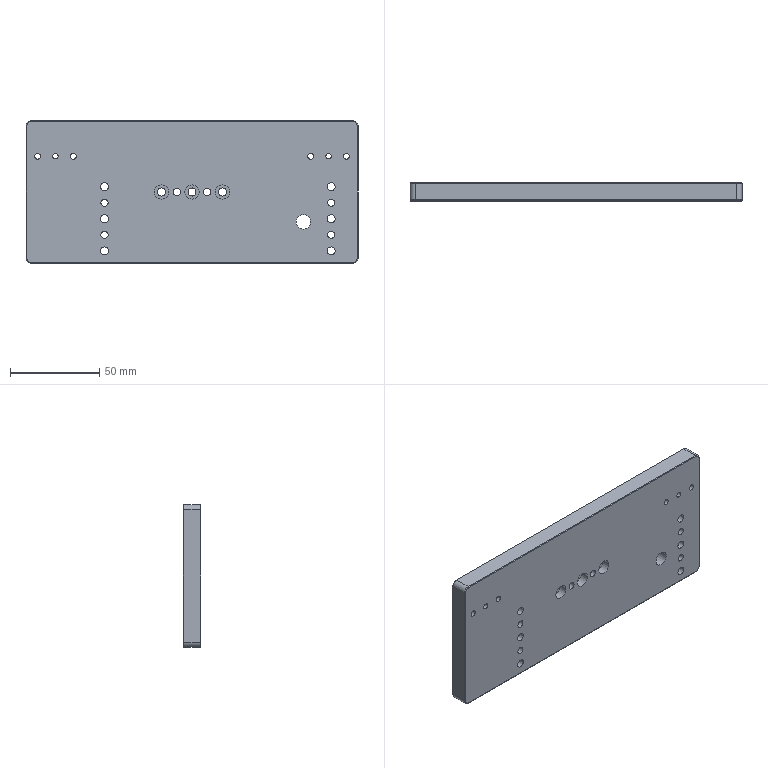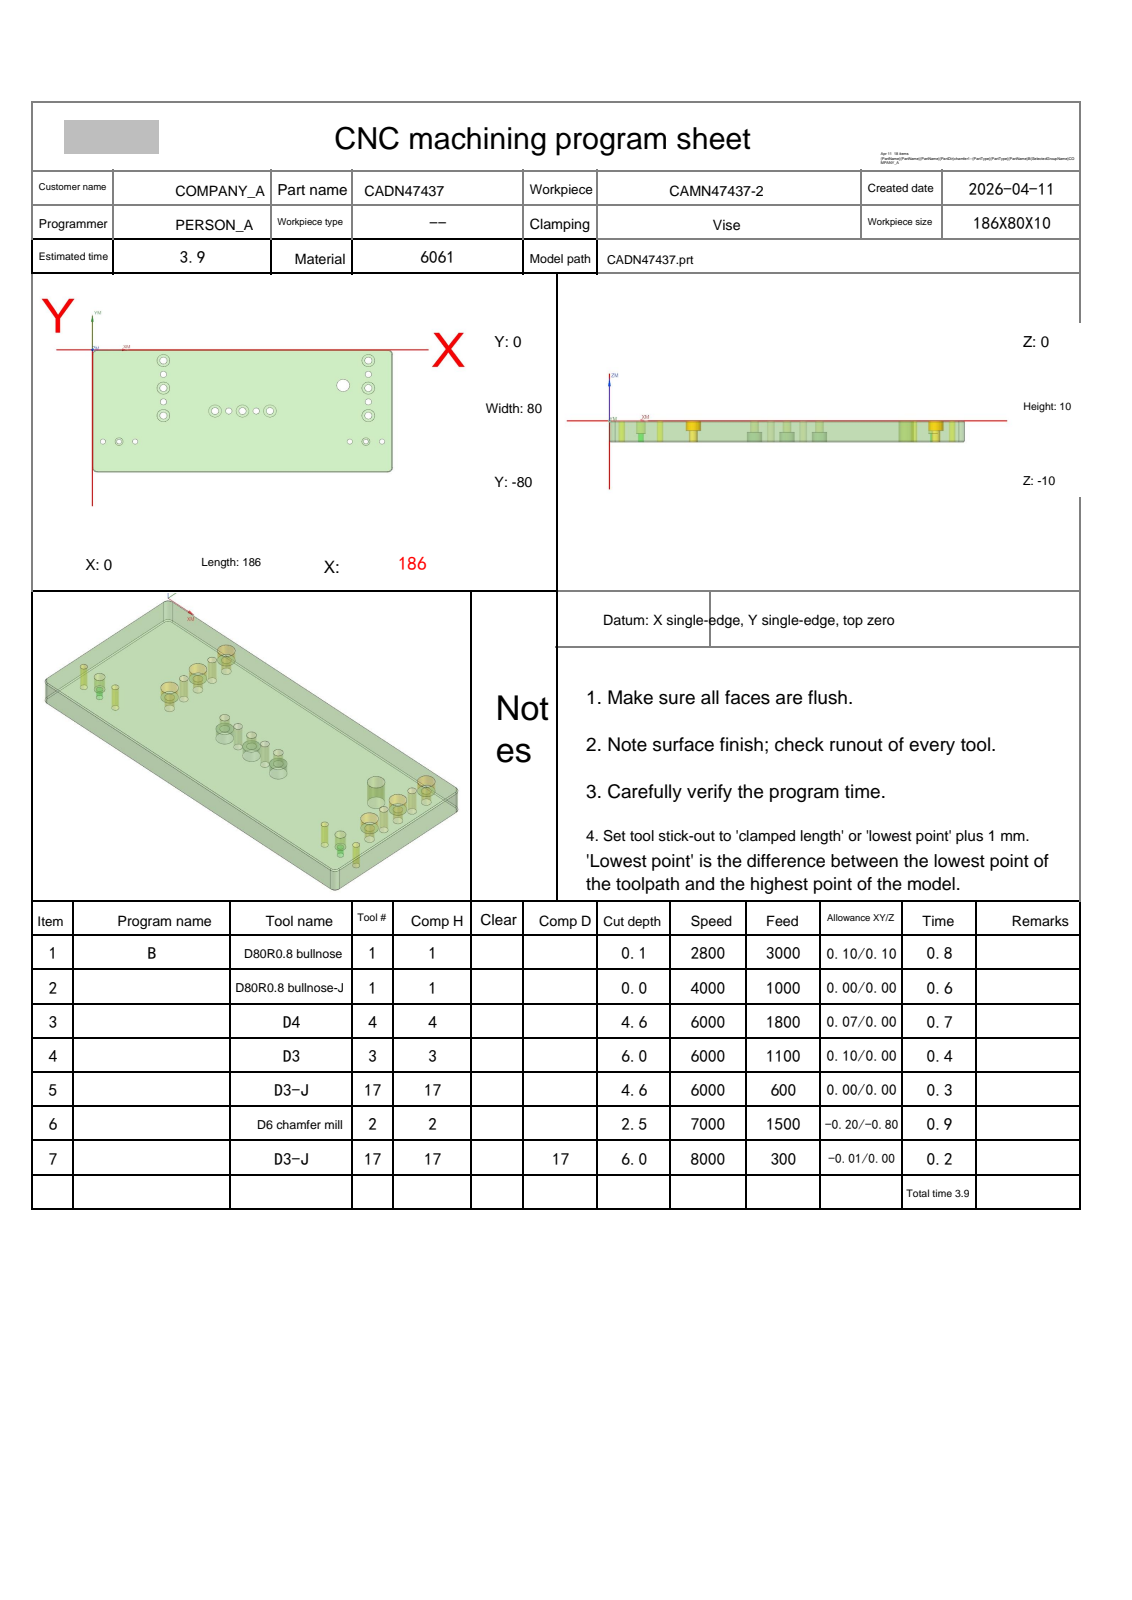NC program | NX | posted by the shop | part box 186 x 10 x 80 mm
Whole program:
%
O0001
(Machine time: 5.17 MIN)
(===Total Tool:5===)
(T1=D80R0.8 bullnose D=80.  R=0.8  D-  H01 Z=0.    )
(T4=D4      D=4.   R=0.   D-  H04 Z=-4.6  )
(T3=D3      D=3.   R=0.   D-  H03 Z=-6.   )
(T17=D3-J   D=3.   R=0.   D-  H17 Z=-6.   )
(T2=D6 chamfer mill   D=6.   R=0.   D-  H02 Z=-2.45 )
G80 G90 G17 G49 G40
G91 G28 Z0
M01
N1 T01 M06
(D80R0.8 bullnose  D=80. R=0.8 H=01 ce=0.10 di=0.10)
G00 G90 G54 X238.097 Y-55.279 M03 S2800
G43 H01 Z20.
M08
Z3.525
G01 Z1.525 F3000.
X226.097 Y-55.457
X-32.79 Y-59.288
X-32.897 Y-59.289
G02 X-40.097 Y-52.089 I0.0 J7.2
G01 Y-39.787
G02 X-32.215 Y-31.788 I8. J0.0
G01 X226.097 Y-27.964
X238.097 Y-27.787
Z3.525
G00 Y-55.279
Z3.05
G01 Z1.05
X226.097 Y-55.457
X-32.79 Y-59.288
X-32.897 Y-59.289
G02 X-40.097 Y-52.089 I0.0 J7.2
G01 Y-39.787
G02 X-32.215 Y-31.788 I8. J0.0
G01 X226.097 Y-27.964
X238.097 Y-27.787
Z3.05
G00 Y-55.279
Z2.575
G01 Z.575
X226.097 Y-55.457
X-32.79 Y-59.288
X-32.897 Y-59.289
G02 X-40.097 Y-52.089 I0.0 J7.2
G01 Y-39.787
G02 X-32.215 Y-31.788 I8. J0.0
G01 X226.097 Y-27.964
X238.097 Y-27.787
Z2.575
G00 Y-55.279
Z2.1
G01 Z.1
X226.097 Y-55.457
X-32.79 Y-59.288
X-32.897 Y-59.289
G02 X-40.097 Y-52.089 I0.0 J7.2
G01 Y-39.787
G02 X-32.215 Y-31.788 I8. J0.0
G01 X226.097 Y-27.964
X238.097 Y-27.787
Z2.1
G00 Z20.
G91 G28 Z0.0
M05
M09
G91 G28 Z0.0
M01
N2 T01 M06
(D80R0.8 bullnose-J  D=80. R=0.8 H=01 ce=0.00 di=0.00)
G00 G90 G54 X237.999 Y-55.182 M03 S4000
G43 H01 Z20.
M08
Z2.
G01 Z0.0 F1000.
X225.999 Y-55.359
X-32.692 Y-59.193
X-32.799
G02 X-39.999 Y-51.993 I0.0 J7.2
G01 Y-39.884
G02 X-32.118 Y-31.885 I8. J0.0
G01 X225.999 Y-28.06
X237.999 Y-27.882
Z2.
G00 Z20.
G91 G28 Z0.0
M05
M09
G91 G28 Z0.0
M01
N3 T04 M06
(D4  D=4. R=0. H=04 ce=0.07 di=0.00)
G00 G90 G54 X171. Y-25. M03 S6000
G43 H04 Z20.
M08
Z.3
G03 X171.965 Y-25.965 I.965 J0.0 F1800.
X172.93 Y-25. I0.0 J.965
X172.93 Y-25. Z-.05 I-1.93 J0.0
X172.93 Y-25. Z-.4 I-1.93 J0.0
X172.93 Y-25. Z-.75 I-1.93 J0.0
X172.93 Y-25. Z-1.1 I-1.93 J0.0
X172.93 Y-25. Z-1.45 I-1.93 J0.0
X172.93 Y-25. Z-1.8 I-1.93 J0.0
X172.93 Y-25. Z-2.15 I-1.93 J0.0
X172.93 Y-25. Z-2.5 I-1.93 J0.0
X172.93 Y-25. Z-2.85 I-1.93 J0.0
X172.93 Y-25. Z-3.2 I-1.93 J0.0
X172.93 Y-25. Z-3.55 I-1.93 J0.0
X172.93 Y-25. Z-3.9 I-1.93 J0.0
X172.93 Y-25. Z-4.25 I-1.93 J0.0
X172.93 Y-25. Z-4.6 I-1.93 J0.0
X171. Y-23.07 I-1.93 J0.0
X169.07 Y-25. I0.0 J-1.93
X171. Y-26.93 I1.93 J0.0
X172.93 Y-25. I0.0 J1.93
X171.965 Y-24.035 I-.965 J0.0
X171. Y-25. I0.0 J-.965
G00 Z20.
Y-43.
Z.3
G03 X171.965 Y-43.965 I.965 J0.0
X172.93 Y-43. I0.0 J.965
X172.93 Y-43. Z-.05 I-1.93 J0.0
X172.93 Y-43. Z-.4 I-1.93 J0.0
X172.93 Y-43. Z-.75 I-1.93 J0.0
X172.93 Y-43. Z-1.1 I-1.93 J0.0
X172.93 Y-43. Z-1.45 I-1.93 J0.0
X172.93 Y-43. Z-1.8 I-1.93 J0.0
X172.93 Y-43. Z-2.15 I-1.93 J0.0
X172.93 Y-43. Z-2.5 I-1.93 J0.0
X172.93 Y-43. Z-2.85 I-1.93 J0.0
X172.93 Y-43. Z-3.2 I-1.93 J0.0
X172.93 Y-43. Z-3.55 I-1.93 J0.0
X172.93 Y-43. Z-3.9 I-1.93 J0.0
X172.93 Y-43. Z-4.25 I-1.93 J0.0
X172.93 Y-43. Z-4.6 I-1.93 J0.0
X171. Y-41.07 I-1.93 J0.0
X169.07 Y-43. I0.0 J-1.93
X171. Y-44.93 I1.93 J0.0
X172.93 Y-43. I0.0 J1.93
X171.965 Y-42.035 I-.965 J0.0
X171. Y-43. I0.0 J-.965
G00 Z20.
Y-7.
Z.3
G03 X171.965 Y-7.965 I.965 J0.0
X172.93 Y-7. I0.0 J.965
X172.93 Y-7. Z-.05 I-1.93 J0.0
X172.93 Y-7. Z-.4 I-1.93 J0.0
X172.93 Y-7. Z-.75 I-1.93 J0.0
X172.93 Y-7. Z-1.1 I-1.93 J0.0
X172.93 Y-7. Z-1.45 I-1.93 J0.0
X172.93 Y-7. Z-1.8 I-1.93 J0.0
X172.93 Y-7. Z-2.15 I-1.93 J0.0
X172.93 Y-7. Z-2.5 I-1.93 J0.0
X172.93 Y-7. Z-2.85 I-1.93 J0.0
X172.93 Y-7. Z-3.2 I-1.93 J0.0
X172.93 Y-7. Z-3.55 I-1.93 J0.0
X172.93 Y-7. Z-3.9 I-1.93 J0.0
X172.93 Y-7. Z-4.25 I-1.93 J0.0
X172.93 Y-7. Z-4.6 I-1.93 J0.0
X171. Y-5.07 I-1.93 J0.0
X169.07 Y-7. I0.0 J-1.93
X171. Y-8.93 I1.93 J0.0
X172.93 Y-7. I0.0 J1.93
X171.965 Y-6.035 I-.965 J0.0
X171. Y-7. I0.0 J-.965
G00 Z20.
X44.
Z.3
G03 X44.965 Y-7.965 I.965 J0.0
X45.93 Y-7. I0.0 J.965
X45.93 Y-7. Z-.05 I-1.93 J0.0
X45.93 Y-7. Z-.4 I-1.93 J0.0
X45.93 Y-7. Z-.75 I-1.93 J0.0
X45.93 Y-7. Z-1.1 I-1.93 J0.0
X45.93 Y-7. Z-1.45 I-1.93 J0.0
X45.93 Y-7. Z-1.8 I-1.93 J0.0
X45.93 Y-7. Z-2.15 I-1.93 J0.0
X45.93 Y-7. Z-2.5 I-1.93 J0.0
X45.93 Y-7. Z-2.85 I-1.93 J0.0
X45.93 Y-7. Z-3.2 I-1.93 J0.0
X45.93 Y-7. Z-3.55 I-1.93 J0.0
X45.93 Y-7. Z-3.9 I-1.93 J0.0
X45.93 Y-7. Z-4.25 I-1.93 J0.0
X45.93 Y-7. Z-4.6 I-1.93 J0.0
X44. Y-5.07 I-1.93 J0.0
X42.07 Y-7. I0.0 J-1.93
X44. Y-8.93 I1.93 J0.0
X45.93 Y-7. I0.0 J1.93
X44.965 Y-6.035 I-.965 J0.0
X44. Y-7. I0.0 J-.965
G00 Z20.
Y-25.
Z.3
G03 X44.965 Y-25.965 I.965 J0.0
X45.93 Y-25. I0.0 J.965
X45.93 Y-25. Z-.05 I-1.93 J0.0
X45.93 Y-25. Z-.4 I-1.93 J0.0
X45.93 Y-25. Z-.75 I-1.93 J0.0
X45.93 Y-25. Z-1.1 I-1.93 J0.0
X45.93 Y-25. Z-1.45 I-1.93 J0.0
X45.93 Y-25. Z-1.8 I-1.93 J0.0
X45.93 Y-25. Z-2.15 I-1.93 J0.0
X45.93 Y-25. Z-2.5 I-1.93 J0.0
X45.93 Y-25. Z-2.85 I-1.93 J0.0
X45.93 Y-25. Z-3.2 I-1.93 J0.0
X45.93 Y-25. Z-3.55 I-1.93 J0.0
X45.93 Y-25. Z-3.9 I-1.93 J0.0
X45.93 Y-25. Z-4.25 I-1.93 J0.0
X45.93 Y-25. Z-4.6 I-1.93 J0.0
X44. Y-23.07 I-1.93 J0.0
X42.07 Y-25. I0.0 J-1.93
X44. Y-26.93 I1.93 J0.0
X45.93 Y-25. I0.0 J1.93
X44.965 Y-24.035 I-.965 J0.0
X44. Y-25. I0.0 J-.965
G00 Z20.
Y-43.
Z.3
G03 X44.965 Y-43.965 I.965 J0.0
X45.93 Y-43. I0.0 J.965
X45.93 Y-43. Z-.05 I-1.93 J0.0
X45.93 Y-43. Z-.4 I-1.93 J0.0
X45.93 Y-43. Z-.75 I-1.93 J0.0
X45.93 Y-43. Z-1.1 I-1.93 J0.0
X45.93 Y-43. Z-1.45 I-1.93 J0.0
X45.93 Y-43. Z-1.8 I-1.93 J0.0
X45.93 Y-43. Z-2.15 I-1.93 J0.0
X45.93 Y-43. Z-2.5 I-1.93 J0.0
X45.93 Y-43. Z-2.85 I-1.93 J0.0
X45.93 Y-43. Z-3.2 I-1.93 J0.0
X45.93 Y-43. Z-3.55 I-1.93 J0.0
X45.93 Y-43. Z-3.9 I-1.93 J0.0
X45.93 Y-43. Z-4.25 I-1.93 J0.0
X45.93 Y-43. Z-4.6 I-1.93 J0.0
X44. Y-41.07 I-1.93 J0.0
X42.07 Y-43. I0.0 J-1.93
X44. Y-44.93 I1.93 J0.0
X45.93 Y-43. I0.0 J1.93
X44.965 Y-42.035 I-.965 J0.0
X44. Y-43. I0.0 J-.965
G00 Z20.
G91 G28 Z0.0
M05
M09
G91 G28 Z0.0
M01
N4 T03 M06
(D3  D=3. R=0. H=03 ce=0.10 di=0.00)
G00 G90 G54 X169.5 Y-60. M03 S6000
G43 H03 Z20.
M08
Z.3
G03 X169.95 Y-60.45 I.45 J0.0 F1100.
X170.4 Y-60. I0.0 J.45
X170.4 Y-60. Z.1 I-.9 J0.0
X170.4 Y-60. Z-.1 I-.9 J0.0
X170.4 Y-60. Z-.3 I-.9 J0.0
X170.4 Y-60. Z-.5 I-.9 J0.0
X170.4 Y-60. Z-.7 I-.9 J0.0
X170.4 Y-60. Z-.9 I-.9 J0.0
X170.4 Y-60. Z-1.1 I-.9 J0.0
X170.4 Y-60. Z-1.3 I-.9 J0.0
X170.4 Y-60. Z-1.5 I-.9 J0.0
X170.4 Y-60. Z-1.7 I-.9 J0.0
X170.4 Y-60. Z-1.9 I-.9 J0.0
X170.4 Y-60. Z-2.1 I-.9 J0.0
X170.4 Y-60. Z-2.3 I-.9 J0.0
X170.4 Y-60. Z-2.5 I-.9 J0.0
X170.4 Y-60. Z-2.7 I-.9 J0.0
X170.4 Y-60. Z-2.9 I-.9 J0.0
X170.4 Y-60. Z-3.1 I-.9 J0.0
X170.4 Y-60. Z-3.3 I-.9 J0.0
X170.4 Y-60. Z-3.5 I-.9 J0.0
X170.4 Y-60. Z-3.7 I-.9 J0.0
X170.4 Y-60. Z-3.9 I-.9 J0.0
X170.4 Y-60. Z-4.1 I-.9 J0.0
X170.4 Y-60. Z-4.3 I-.9 J0.0
X170.4 Y-60. Z-4.5 I-.9 J0.0
X170.4 Y-60. Z-4.7 I-.9 J0.0
X170.4 Y-60. Z-4.9 I-.9 J0.0
X170.4 Y-60. Z-5.1 I-.9 J0.0
X170.4 Y-60. Z-5.3 I-.9 J0.0
X170.4 Y-60. Z-5.5 I-.9 J0.0
X170.4 Y-60. Z-5.7 I-.9 J0.0
X170.4 Y-60. Z-5.9 I-.9 J0.0
X168.6 Y-60. Z-6. I-.9 J0.0
X169.5 Y-60.9 I.9 J0.0
X170.4 Y-60. I0.0 J.9
X169.5 Y-59.1 I-.9 J0.0
X168.6 Y-60. I0.0 J-.9
X169.05 Y-60.45 I.45 J0.0
X169.5 Y-60. I0.0 J.45
G00 Z20.
X16.5
Z.3
G03 X16.95 Y-60.45 I.45 J0.0
X17.4 Y-60. I0.0 J.45
X17.4 Y-60. Z.1 I-.9 J0.0
X17.4 Y-60. Z-.1 I-.9 J0.0
X17.4 Y-60. Z-.3 I-.9 J0.0
X17.4 Y-60. Z-.5 I-.9 J0.0
X17.4 Y-60. Z-.7 I-.9 J0.0
X17.4 Y-60. Z-.9 I-.9 J0.0
X17.4 Y-60. Z-1.1 I-.9 J0.0
X17.4 Y-60. Z-1.3 I-.9 J0.0
X17.4 Y-60. Z-1.5 I-.9 J0.0
X17.4 Y-60. Z-1.7 I-.9 J0.0
X17.4 Y-60. Z-1.9 I-.9 J0.0
X17.4 Y-60. Z-2.1 I-.9 J0.0
X17.4 Y-60. Z-2.3 I-.9 J0.0
X17.4 Y-60. Z-2.5 I-.9 J0.0
X17.4 Y-60. Z-2.7 I-.9 J0.0
X17.4 Y-60. Z-2.9 I-.9 J0.0
X17.4 Y-60. Z-3.1 I-.9 J0.0
X17.4 Y-60. Z-3.3 I-.9 J0.0
X17.4 Y-60. Z-3.5 I-.9 J0.0
X17.4 Y-60. Z-3.7 I-.9 J0.0
X17.4 Y-60. Z-3.9 I-.9 J0.0
X17.4 Y-60. Z-4.1 I-.9 J0.0
X17.4 Y-60. Z-4.3 I-.9 J0.0
X17.4 Y-60. Z-4.5 I-.9 J0.0
X17.4 Y-60. Z-4.7 I-.9 J0.0
X17.4 Y-60. Z-4.9 I-.9 J0.0
X17.4 Y-60. Z-5.1 I-.9 J0.0
X17.4 Y-60. Z-5.3 I-.9 J0.0
X17.4 Y-60. Z-5.5 I-.9 J0.0
X17.4 Y-60. Z-5.7 I-.9 J0.0
X17.4 Y-60. Z-5.9 I-.9 J0.0
X15.6 Y-60. Z-6. I-.9 J0.0
X16.5 Y-60.9 I.9 J0.0
X17.4 Y-60. I0.0 J.9
X16.5 Y-59.1 I-.9 J0.0
X15.6 Y-60. I0.0 J-.9
X16.05 Y-60.45 I.45 J0.0
X16.5 Y-60. I0.0 J.45
G00 Z20.
G91 G28 Z0.0
M05
M09
G91 G28 Z0.0
M01
N5 T17 M06
(D3-J  D=3. R=0. H=17 ce=0.00 di=0.00)
G00 G90 G54 X171. Y-25. M03 S6000
G43 H17 Z20.
M08
Z-4.6
G01 X173.103 Y-25.338 F600.
X173.157 Y-25.343
G03 X173.5 Y-25. I0.0 J.343
X171. Y-22.5 I-2.5 J0.0
X168.5 Y-25. I0.0 J-2.5
X171. Y-27.5 I2.5 J0.0
X173.5 Y-25. I0.0 J2.5
X173.45 Y-24.503 I-2.5 J0.0
X173.114 Y-24.229 I-.336 J-.068
G01 X172.994 Y-24.251
X171. Y-25.
G00 Z20.
Y-43.
Z-4.6
G01 X173.103 Y-43.338
X173.157 Y-43.343
G03 X173.5 Y-43. I0.0 J.343
X171. Y-40.5 I-2.5 J0.0
X168.5 Y-43. I0.0 J-2.5
X171. Y-45.5 I2.5 J0.0
X173.5 Y-43. I0.0 J2.5
X173.45 Y-42.503 I-2.5 J0.0
X173.114 Y-42.229 I-.336 J-.068
G01 X172.994 Y-42.251
X171. Y-43.
G00 Z20.
Y-7.
Z-4.6
G01 X173.103 Y-7.338
X173.157 Y-7.343
G03 X173.5 Y-7. I0.0 J.343
X171. Y-4.5 I-2.5 J0.0
X168.5 Y-7. I0.0 J-2.5
X171. Y-9.5 I2.5 J0.0
X173.5 Y-7. I0.0 J2.5
X173.45 Y-6.503 I-2.5 J0.0
X173.114 Y-6.229 I-.336 J-.068
G01 X172.994 Y-6.251
X171. Y-7.
G00 Z20.
X44.
Z-4.6
G01 X46.103 Y-7.338
X46.157 Y-7.343
G03 X46.5 Y-7. I0.0 J.343
X44. Y-4.5 I-2.5 J0.0
X41.5 Y-7. I0.0 J-2.5
X44. Y-9.5 I2.5 J0.0
X46.5 Y-7. I0.0 J2.5
X46.45 Y-6.503 I-2.5 J0.0
X46.114 Y-6.229 I-.336 J-.068
G01 X45.994 Y-6.251
X44. Y-7.
G00 Z20.
Y-25.
Z-4.6
G01 X46.103 Y-25.338
X46.157 Y-25.343
G03 X46.5 Y-25. I0.0 J.343
X44. Y-22.5 I-2.5 J0.0
X41.5 Y-25. I0.0 J-2.5
X44. Y-27.5 I2.5 J0.0
X46.5 Y-25. I0.0 J2.5
X46.45 Y-24.503 I-2.5 J0.0
X46.114 Y-24.229 I-.336 J-.068
G01 X45.994 Y-24.251
X44. Y-25.
G00 Z20.
Y-43.
Z-4.6
G01 X46.103 Y-43.338
X46.157 Y-43.343
G03 X46.5 Y-43. I0.0 J.343
X44. Y-40.5 I-2.5 J0.0
X41.5 Y-43. I0.0 J-2.5
X44. Y-45.5 I2.5 J0.0
X46.5 Y-43. I0.0 J2.5
X46.45 Y-42.503 I-2.5 J0.0
X46.114 Y-42.229 I-.336 J-.068
G01 X45.994 Y-42.251
X44. Y-43.
G00 Z20.
G91 G28 Z0.0
M05
M09
G91 G28 Z0.0
M01
N6 T02 M06
(D6 chamfer mill  D=6. R=0. H=02 ce=0.00 di=0.00)
G00 G90 G54 X6.5 Y-60. M03 S7000
G43 H02 Z20.
M08
G98 G81 X6.5 Y-60. Z-2.2 R3. F500.
X26.5
X159.5
X179.5
G80
G00 Z20.
G00 G90 X44. Y-16. M03 S7000
Z20.
G98 G81 X44. Y-16. Z-2.2 R3. F500.
Y-34.
X84.5 Y-40.
X101.5
X171. Y-34.
Y-16.
G80
G00 Z20.
G00 G90 X110. Y-40. M03 S7000
Z20.
G98 G81 X110. Y-40. Z-2.45 R3. F500.
X93.
X76.
G80
G00 Z20.
G00 G90 X168.806 Y-60.093 M03 S7000
Z20.
Z-.5
G01 Z-1. F600.
X168. Y-60.2
G03 X169.5 Y-61.7 I1.5 J0.0
X171.2 Y-60. I0.0 J1.7
X169.5 Y-58.3 I-1.7 J0.0
X167.8 Y-60. I0.0 J-1.7
X169.5 Y-61.7 I1.7 J0.0
X171. Y-60.2 I0.0 J1.5
G01 X170.194 Y-60.093
Z-.5
G00 Z20.
X15.806
Z-.5
G01 Z-1.
X15. Y-60.2
G03 X16.5 Y-61.7 I1.5 J0.0
X18.2 Y-60. I0.0 J1.7
X16.5 Y-58.3 I-1.7 J0.0
X14.8 Y-60. I0.0 J-1.7
X16.5 Y-61.7 I1.7 J0.0
X18. Y-60.2 I0.0 J1.5
G01 X17.194 Y-60.093
Z-.5
G00 Z20.
G00 G90 X42.913 Y-7.507 M03 S7000
Z20.
Z-1.5
G01 Z-2. F600.
X42.5 Y-7.7
G03 X44. Y-9.2 I1.5 J0.0
X46.2 Y-7. I0.0 J2.2
X44. Y-4.8 I-2.2 J0.0
X41.8 Y-7. I0.0 J-2.2
X44. Y-9.2 I2.2 J0.0
X45.5 Y-7.7 I0.0 J1.5
G01 X45.087 Y-7.507
Z-1.5
G00 Z20.
X42.913 Y-25.507
Z-1.5
G01 Z-2.
X42.5 Y-25.7
G03 X44. Y-27.2 I1.5 J0.0
X46.2 Y-25. I0.0 J2.2
X44. Y-22.8 I-2.2 J0.0
X41.8 Y-25. I0.0 J-2.2
X44. Y-27.2 I2.2 J0.0
X45.5 Y-25.7 I0.0 J1.5
G01 X45.087 Y-25.507
Z-1.5
G00 Z20.
X42.913 Y-43.507
Z-1.5
G01 Z-2.
X42.5 Y-43.7
G03 X44. Y-45.2 I1.5 J0.0
X46.2 Y-43. I0.0 J2.2
X44. Y-40.8 I-2.2 J0.0
X41.8 Y-43. I0.0 J-2.2
X44. Y-45.2 I2.2 J0.0
X45.5 Y-43.7 I0.0 J1.5
G01 X45.087 Y-43.507
Z-1.5
G00 Z20.
X169.913
Z-1.5
G01 Z-2.
X169.5 Y-43.7
G03 X171. Y-45.2 I1.5 J0.0
X173.2 Y-43. I0.0 J2.2
X171. Y-40.8 I-2.2 J0.0
X168.8 Y-43. I0.0 J-2.2
X171. Y-45.2 I2.2 J0.0
X172.5 Y-43.7 I0.0 J1.5
G01 X172.087 Y-43.507
Z-1.5
G00 Z20.
X169.913 Y-25.507
Z-1.5
G01 Z-2.
X169.5 Y-25.7
G03 X171. Y-27.2 I1.5 J0.0
X173.2 Y-25. I0.0 J2.2
X171. Y-22.8 I-2.2 J0.0
X168.8 Y-25. I0.0 J-2.2
X171. Y-27.2 I2.2 J0.0
X172.5 Y-25.7 I0.0 J1.5
G01 X172.087 Y-25.507
Z-1.5
G00 Z20.
X169.913 Y-7.507
Z-1.5
G01 Z-2.
X169.5 Y-7.7
G03 X171. Y-9.2 I1.5 J0.0
X173.2 Y-7. I0.0 J2.2
X171. Y-4.8 I-2.2 J0.0
X168.8 Y-7. I0.0 J-2.2
X171. Y-9.2 I2.2 J0.0
X172.5 Y-7.7 I0.0 J1.5
G01 X172.087 Y-7.507
Z-1.5
G00 Z20.
G00 G90 X153.901 Y-24.245 M03 S7000
Z20.
Z-.9
G01 Z-1.4 F600.
Y-24.55
G03 X155.401 Y-26.05 I1.5 J0.0
X158.201 Y-23.25 I0.0 J2.8
X155.401 Y-20.45 I-2.8 J0.0
X152.601 Y-23.25 I0.0 J-2.8
X155.401 Y-26.05 I2.8 J0.0
X156.901 Y-24.55 I0.0 J1.5
G01 Y-24.245
Z-.9
G00 Z20.
G00 G90 X1.809 Y1.753 M03 S6500
Z20.
Z.3
G01 Z-1.2 F1500.
G03 X3. Y.7 I1.191 J.147
G01 X183.
G02 X186.7 Y-3. I0.0 J-3.7
G01 Y-77.
G02 X183. Y-80.7 I-3.7 J0.0
G01 X3.
G02 X-.7 Y-77. I0.0 J3.7
G01 Y-3.
G02 X3. Y.7 I3.7 J0.0
G01 X3.4
G03 X4.6 Y1.9 I0.0 J1.2
G01 Z.3
G00 Z20.
G91 G28 Z0.0
M05
M09
G91 G28 Z0.0
M01
N7 T17 M06
(D3-J  D=3. R=0. H=17 ce=-0.01 di=0.00)
G00 G90 G54 X16.264 Y-59.659 M03 S8000
G43 H17 Z11.8
M08
Z-2.
G01 Z-3. F300.
G41 D17
X16.085 Y-59.4
G03 X15.485 Y-60. I0.0 J-.6
X16.5 Y-61.015 I1.015 J0.0
X17.515 Y-60. I0.0 J1.015
X16.5 Y-58.985 I-1.015 J0.0
X15.485 Y-60. I0.0 J-1.015
X15.563 Y-60.39 I1.015 J0.0
X16.117 Y-60.759 I.554 J.23
X16.347 Y-60.713 I0.0 J.6
G01 G40 X16.413 Y-60.406
Z-2.
G00 X16.264 Y-59.659
Z-5.
G01 Z-6.
G41 D17
X16.085 Y-59.4
G03 X15.485 Y-60. I0.0 J-.6
X16.5 Y-61.015 I1.015 J0.0
X17.515 Y-60. I0.0 J1.015
X16.5 Y-58.985 I-1.015 J0.0
X15.485 Y-60. I0.0 J-1.015
X15.563 Y-60.39 I1.015 J0.0
X16.117 Y-60.759 I.554 J.23
X16.347 Y-60.713 I0.0 J.6
G01 G40 X16.413 Y-60.406
Z-5.
G00 Z11.8
X169.736 Y-60.341
Z-2.
G01 Z-3.
G41 D17
X169.915 Y-60.6
G03 X170.515 Y-60. I0.0 J.6
X169.5 Y-58.985 I-1.015 J0.0
X168.485 Y-60. I0.0 J-1.015
X169.5 Y-61.015 I1.015 J0.0
X170.515 Y-60. I0.0 J1.015
X170.437 Y-59.61 I-1.015 J0.0
X169.883 Y-59.241 I-.554 J-.23
X169.653 Y-59.287 I0.0 J-.6
G01 G40 X169.587 Y-59.594
Z-2.
G00 X169.736 Y-60.341
Z-5.
G01 Z-6.
G41 D17
X169.915 Y-60.6
G03 X170.515 Y-60. I0.0 J.6
X169.5 Y-58.985 I-1.015 J0.0
X168.485 Y-60. I0.0 J-1.015
X169.5 Y-61.015 I1.015 J0.0
X170.515 Y-60. I0.0 J1.015
X170.437 Y-59.61 I-1.015 J0.0
X169.883 Y-59.241 I-.554 J-.23
X169.653 Y-59.287 I0.0 J-.6
G01 G40 X169.587 Y-59.594
Z-5.
G00 Z11.8
M05
M09
G91 G28 Z0.0
G91 G28 Y0.0
M30
%